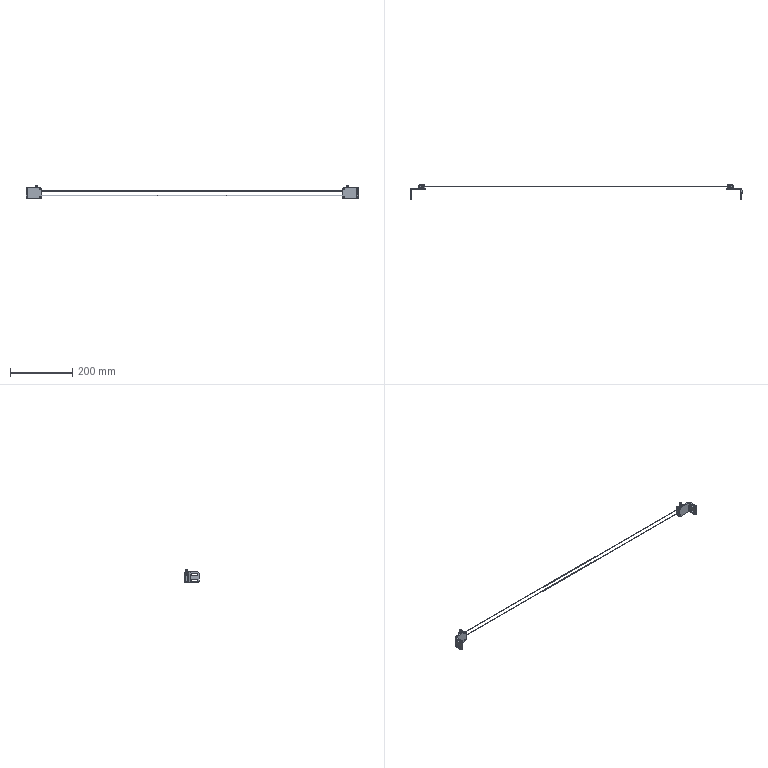Part | SolidWorks | 4 solids | 1034 faces | box 1070 x 46.001 x 43.6 mm | volume 37995 mm3 | plane 382 | cylinder 320 | spline 126 | torus 104 | cone 62 | sphere 40 | commonest cylinder face diameters 0.2 x136 0.6 x28 1 x24 6 x16 2.4 x12 3.6 x12